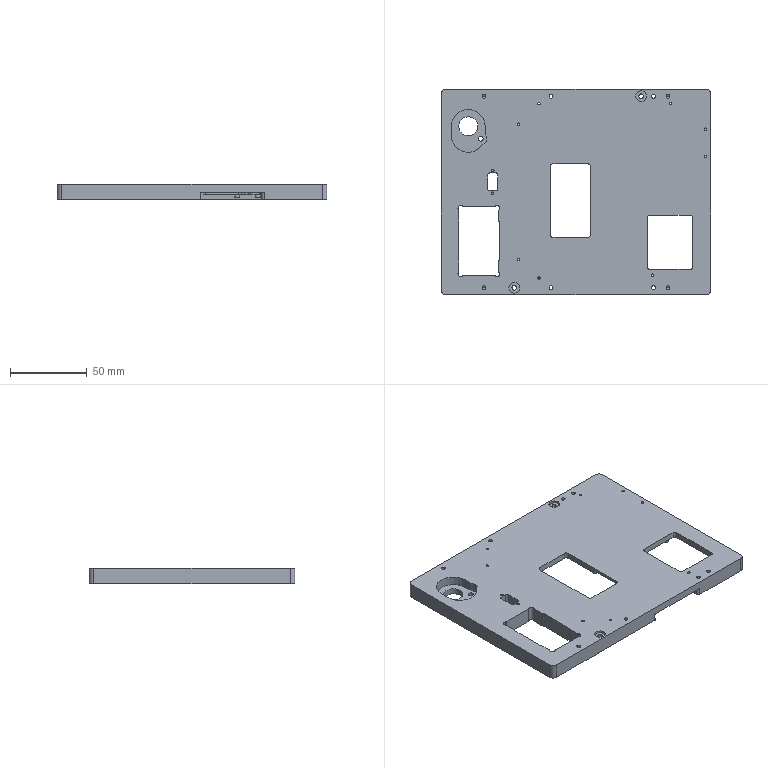NC program | NX | posted with a generic post | part box 176 x 134 x 10 mm
Lines 1 to 97 of 17594:
N10 G17 G21 G94 G90
(FLOOR_WALL_COPY_COPY , TOOL : D63)
N12 T03 M6
N14 G54
N16 G17 G0 G90 X-122.5 Y66.999 S6500 M3
N18 G43 Z30. H3
N20 Z7.02
N22 G94 G1 Z4.02 F1250.
N24 X-119.5
N26 X119.5
N28 Y30.733
N30 X-119.5
N32 Y-5.534
N34 X119.5
N36 Y-41.8
N38 X-119.5
N40 X-122.5
N42 Z7.02
N44 G0 Z30.
N46 Y66.999
N48 Z6.04
N50 G1 Z3.04
N52 X-119.5
N54 X119.5
N56 Y30.733
N58 X-119.5
N60 Y-5.534
N62 X119.5
N64 Y-41.8
N66 X-119.5
N68 X-122.5
N70 Z6.04
N72 G0 Z30.
N74 Y66.999
N76 Z5.06
N78 G1 Z2.06
N80 X-119.5
N82 X119.5
N84 Y30.733
N86 X-119.5
N88 Y-5.534
N90 X119.5
N92 Y-41.8
N94 X-119.5
N96 X-122.5
N98 Z5.06
N100 G0 Z30.
N102 Y66.999
N104 Z4.08
N106 G1 Z1.08
N108 X-119.5
N110 X119.5
N112 Y30.733
N114 X-119.5
N116 Y-5.534
N118 X119.5
N120 Y-41.8
N122 X-119.5
N124 X-122.5
N126 Z4.08
N128 G0 Z30.
N130 Y66.999
N132 Z3.1
N134 G1 Z0.1
N136 X-119.5
N138 X119.5
N140 Y30.733
N142 X-119.5
N144 Y-5.534
N146 X119.5
N148 Y-41.8
N150 X-119.5
N152 X-122.5
N154 Z3.1
N156 G0 Z30.
(FLOOR_WALL_COPY_COPY_1 , TOOL : D63)
N158 Y66.999
N160 Z3.
N162 G1 Z0.
N164 X-119.5
N166 X119.5
N168 Y30.733
N170 X-119.5
N172 Y-5.534
N174 X119.5
N176 Y-41.8
N178 X-119.5
N180 X-122.5
N182 Z3.
N184 G0 Z30.
N186 M5